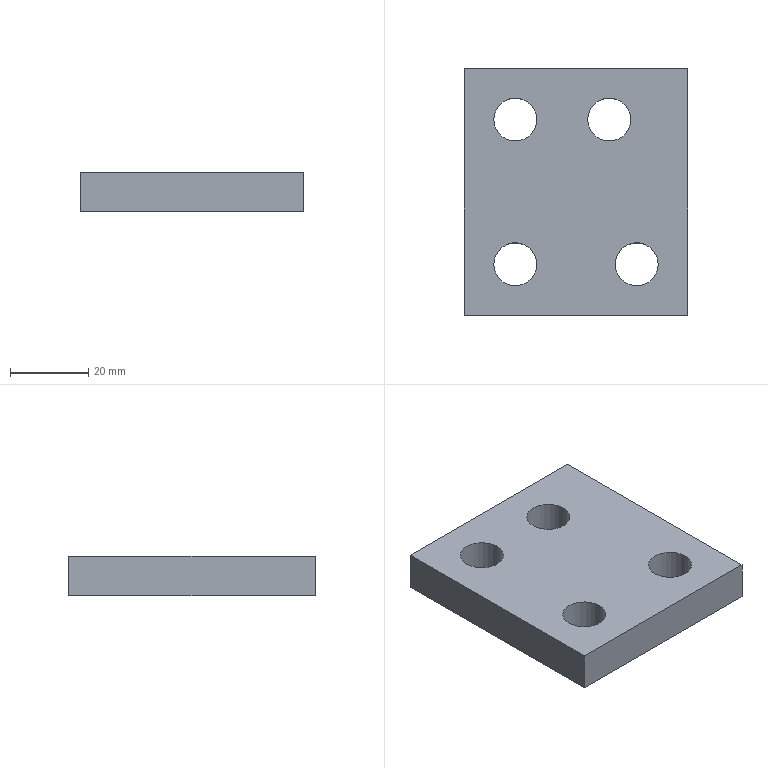Part | NX | features solid 2 | 1 solid | 10 faces | box 57 x 63 x 10 mm | volume 32109 mm3 | plane 6 | cylinder 4 | commonest cylinder face diameters 11 x4
STEP:
#1=CARTESIAN_POINT('',(139.,121.5,88.));
#2=VERTEX_POINT('',#1);
#3=CARTESIAN_POINT('',(133.5,121.5,88.));
#4=DIRECTION('',(0.,0.,1.));
#5=DIRECTION('',(1.,0.,0.));
#6=AXIS2_PLACEMENT_3D('',#3,#4,#5);
#7=CIRCLE('',#6,5.5);
#8=EDGE_CURVE('',#2,#2,#7,.T.);
#9=ORIENTED_EDGE('',*,*,#8,.F.);
#10=EDGE_LOOP('',(#9));
#11=FACE_BOUND('',#10,.T.);
#12=CARTESIAN_POINT('',(163.,158.5,88.));
#13=VERTEX_POINT('',#12);
#14=CARTESIAN_POINT('',(157.5,158.5,88.));
#15=DIRECTION('',(0.,0.,1.));
#16=DIRECTION('',(1.,0.,0.));
#17=AXIS2_PLACEMENT_3D('',#14,#15,#16);
#18=CIRCLE('',#17,5.5);
#19=EDGE_CURVE('',#13,#13,#18,.T.);
#20=ORIENTED_EDGE('',*,*,#19,.F.);
#21=EDGE_LOOP('',(#20));
#22=FACE_BOUND('',#21,.T.);
#23=CARTESIAN_POINT('',(139.,158.5,88.));
#24=VERTEX_POINT('',#23);
#25=CARTESIAN_POINT('',(133.5,158.5,88.));
#26=DIRECTION('',(0.,0.,1.));
#27=DIRECTION('',(1.,0.,0.));
#28=AXIS2_PLACEMENT_3D('',#25,#26,#27);
#29=CIRCLE('',#28,5.5);
#30=EDGE_CURVE('',#24,#24,#29,.T.);
#31=ORIENTED_EDGE('',*,*,#30,.F.);
#32=EDGE_LOOP('',(#31));
#33=FACE_BOUND('',#32,.T.);
#34=CARTESIAN_POINT('',(170.,121.5,88.));
#35=VERTEX_POINT('',#34);
#36=CARTESIAN_POINT('',(164.5,121.5,88.));
#37=DIRECTION('',(0.,0.,1.));
#38=DIRECTION('',(1.,0.,0.));
#39=AXIS2_PLACEMENT_3D('',#36,#37,#38);
#40=CIRCLE('',#39,5.5);
#41=EDGE_CURVE('',#35,#35,#40,.T.);
#42=ORIENTED_EDGE('',*,*,#41,.F.);
#43=EDGE_LOOP('',(#42));
#44=FACE_BOUND('',#43,.T.);
#45=CARTESIAN_POINT('',(177.5,108.5,88.));
#46=VERTEX_POINT('',#45);
#47=CARTESIAN_POINT('',(120.5,108.5,88.));
#48=VERTEX_POINT('',#47);
#49=CARTESIAN_POINT('',(149.,108.5,88.));
#50=DIRECTION('',(-1.,0.,0.));
#51=VECTOR('',#50,1000.);
#52=LINE('',#49,#51);
#53=EDGE_CURVE('',#46,#48,#52,.T.);
#54=ORIENTED_EDGE('',*,*,#53,.F.);
#55=CARTESIAN_POINT('',(177.5,171.5,88.));
#56=VERTEX_POINT('',#55);
#57=CARTESIAN_POINT('',(177.5,140.,88.));
#58=DIRECTION('',(0.,-1.,0.));
#59=VECTOR('',#58,1000.);
#60=LINE('',#57,#59);
#61=EDGE_CURVE('',#56,#46,#60,.T.);
#62=ORIENTED_EDGE('',*,*,#61,.F.);
#63=CARTESIAN_POINT('',(120.5,171.5,88.));
#64=VERTEX_POINT('',#63);
#65=CARTESIAN_POINT('',(149.,171.5,88.));
#66=DIRECTION('',(1.,0.,0.));
#67=VECTOR('',#66,1000.);
#68=LINE('',#65,#67);
#69=EDGE_CURVE('',#64,#56,#68,.T.);
#70=ORIENTED_EDGE('',*,*,#69,.F.);
#71=CARTESIAN_POINT('',(120.5,140.,88.));
#72=DIRECTION('',(0.,1.,0.));
#73=VECTOR('',#72,1000.);
#74=LINE('',#71,#73);
#75=EDGE_CURVE('',#48,#64,#74,.T.);
#76=ORIENTED_EDGE('',*,*,#75,.F.);
#77=EDGE_LOOP('',(#54,#62,#70,#76));
#78=FACE_BOUND('',#77,.T.);
#79=CARTESIAN_POINT('',(268.879,280.,88.));
#80=DIRECTION('',(0.,0.,1.));
#81=DIRECTION('',(-1.,0.,0.));
#82=AXIS2_PLACEMENT_3D('',#79,#80,#81);
#83=PLANE('',#82);
#84=ADVANCED_FACE('',(#11,#22,#33,#44,#78),#83,.T.);
#85=CARTESIAN_POINT('',(177.5,108.5,78.));
#86=VERTEX_POINT('',#85);
#87=CARTESIAN_POINT('',(177.5,108.5,19.));
#88=DIRECTION('',(0.,0.,1.));
#89=VECTOR('',#88,1000.);
#90=LINE('',#87,#89);
#91=EDGE_CURVE('',#86,#46,#90,.T.);
#92=ORIENTED_EDGE('',*,*,#91,.T.);
#93=ORIENTED_EDGE('',*,*,#53,.T.);
#94=CARTESIAN_POINT('',(120.5,108.5,78.));
#95=VERTEX_POINT('',#94);
#96=CARTESIAN_POINT('',(120.5,108.5,19.));
#97=DIRECTION('',(0.,0.,1.));
#98=VECTOR('',#97,1000.);
#99=LINE('',#96,#98);
#100=EDGE_CURVE('',#95,#48,#99,.T.);
#101=ORIENTED_EDGE('',*,*,#100,.F.);
#102=CARTESIAN_POINT('',(149.,108.5,78.));
#103=DIRECTION('',(1.,0.,0.));
#104=VECTOR('',#103,1000.);
#105=LINE('',#102,#104);
#106=EDGE_CURVE('',#95,#86,#105,.T.);
#107=ORIENTED_EDGE('',*,*,#106,.T.);
#108=EDGE_LOOP('',(#92,#93,#101,#107));
#109=FACE_BOUND('',#108,.T.);
#110=CARTESIAN_POINT('',(149.,108.5,19.));
#111=DIRECTION('',(0.,-1.,0.));
#112=DIRECTION('',(0.,0.,-1.));
#113=AXIS2_PLACEMENT_3D('',#110,#111,#112);
#114=PLANE('',#113);
#115=ADVANCED_FACE('',(#109),#114,.T.);
#116=ORIENTED_EDGE('',*,*,#100,.T.);
#117=ORIENTED_EDGE('',*,*,#75,.T.);
#118=CARTESIAN_POINT('',(120.5,171.5,78.));
#119=VERTEX_POINT('',#118);
#120=CARTESIAN_POINT('',(120.5,171.5,19.));
#121=DIRECTION('',(0.,0.,1.));
#122=VECTOR('',#121,1000.);
#123=LINE('',#120,#122);
#124=EDGE_CURVE('',#119,#64,#123,.T.);
#125=ORIENTED_EDGE('',*,*,#124,.F.);
#126=CARTESIAN_POINT('',(120.5,140.,78.));
#127=DIRECTION('',(0.,-1.,0.));
#128=VECTOR('',#127,1000.);
#129=LINE('',#126,#128);
#130=EDGE_CURVE('',#119,#95,#129,.T.);
#131=ORIENTED_EDGE('',*,*,#130,.T.);
#132=EDGE_LOOP('',(#116,#117,#125,#131));
#133=FACE_BOUND('',#132,.T.);
#134=CARTESIAN_POINT('',(120.5,140.,19.));
#135=DIRECTION('',(-1.,0.,0.));
#136=DIRECTION('',(0.,0.,1.));
#137=AXIS2_PLACEMENT_3D('',#134,#135,#136);
#138=PLANE('',#137);
#139=ADVANCED_FACE('',(#133),#138,.T.);
#140=ORIENTED_EDGE('',*,*,#124,.T.);
#141=ORIENTED_EDGE('',*,*,#69,.T.);
#142=CARTESIAN_POINT('',(177.5,171.5,78.));
#143=VERTEX_POINT('',#142);
#144=CARTESIAN_POINT('',(177.5,171.5,19.));
#145=DIRECTION('',(0.,0.,1.));
#146=VECTOR('',#145,1000.);
#147=LINE('',#144,#146);
#148=EDGE_CURVE('',#143,#56,#147,.T.);
#149=ORIENTED_EDGE('',*,*,#148,.F.);
#150=CARTESIAN_POINT('',(149.,171.5,78.));
#151=DIRECTION('',(-1.,0.,0.));
#152=VECTOR('',#151,1000.);
#153=LINE('',#150,#152);
#154=EDGE_CURVE('',#143,#119,#153,.T.);
#155=ORIENTED_EDGE('',*,*,#154,.T.);
#156=EDGE_LOOP('',(#140,#141,#149,#155));
#157=FACE_BOUND('',#156,.T.);
#158=CARTESIAN_POINT('',(149.,171.5,19.));
#159=DIRECTION('',(0.,1.,0.));
#160=DIRECTION('',(0.,0.,1.));
#161=AXIS2_PLACEMENT_3D('',#158,#159,#160);
#162=PLANE('',#161);
#163=ADVANCED_FACE('',(#157),#162,.T.);
#164=CARTESIAN_POINT('',(139.,121.5,78.));
#165=VERTEX_POINT('',#164);
#166=CARTESIAN_POINT('',(133.5,121.5,78.));
#167=DIRECTION('',(0.,0.,1.));
#168=DIRECTION('',(1.,0.,0.));
#169=AXIS2_PLACEMENT_3D('',#166,#167,#168);
#170=CIRCLE('',#169,5.5);
#171=EDGE_CURVE('',#165,#165,#170,.T.);
#172=ORIENTED_EDGE('',*,*,#171,.T.);
#173=EDGE_LOOP('',(#172));
#174=FACE_BOUND('',#173,.T.);
#175=CARTESIAN_POINT('',(163.,158.5,78.));
#176=VERTEX_POINT('',#175);
#177=CARTESIAN_POINT('',(157.5,158.5,78.));
#178=DIRECTION('',(0.,0.,1.));
#179=DIRECTION('',(1.,0.,0.));
#180=AXIS2_PLACEMENT_3D('',#177,#178,#179);
#181=CIRCLE('',#180,5.5);
#182=EDGE_CURVE('',#176,#176,#181,.T.);
#183=ORIENTED_EDGE('',*,*,#182,.T.);
#184=EDGE_LOOP('',(#183));
#185=FACE_BOUND('',#184,.T.);
#186=CARTESIAN_POINT('',(139.,158.5,78.));
#187=VERTEX_POINT('',#186);
#188=CARTESIAN_POINT('',(133.5,158.5,78.));
#189=DIRECTION('',(0.,0.,1.));
#190=DIRECTION('',(1.,0.,0.));
#191=AXIS2_PLACEMENT_3D('',#188,#189,#190);
#192=CIRCLE('',#191,5.5);
#193=EDGE_CURVE('',#187,#187,#192,.T.);
#194=ORIENTED_EDGE('',*,*,#193,.T.);
#195=EDGE_LOOP('',(#194));
#196=FACE_BOUND('',#195,.T.);
#197=CARTESIAN_POINT('',(170.,121.5,78.));
#198=VERTEX_POINT('',#197);
#199=CARTESIAN_POINT('',(164.5,121.5,78.));
#200=DIRECTION('',(0.,0.,1.));
#201=DIRECTION('',(1.,0.,0.));
#202=AXIS2_PLACEMENT_3D('',#199,#200,#201);
#203=CIRCLE('',#202,5.5);
#204=EDGE_CURVE('',#198,#198,#203,.T.);
#205=ORIENTED_EDGE('',*,*,#204,.T.);
#206=EDGE_LOOP('',(#205));
#207=FACE_BOUND('',#206,.T.);
#208=CARTESIAN_POINT('',(177.5,140.,78.));
#209=DIRECTION('',(0.,1.,0.));
#210=VECTOR('',#209,1000.);
#211=LINE('',#208,#210);
#212=EDGE_CURVE('',#86,#143,#211,.T.);
#213=ORIENTED_EDGE('',*,*,#212,.F.);
#214=ORIENTED_EDGE('',*,*,#106,.F.);
#215=ORIENTED_EDGE('',*,*,#130,.F.);
#216=ORIENTED_EDGE('',*,*,#154,.F.);
#217=EDGE_LOOP('',(#213,#214,#215,#216));
#218=FACE_BOUND('',#217,.T.);
#219=CARTESIAN_POINT('',(149.,140.,78.));
#220=DIRECTION('',(0.,0.,-1.));
#221=DIRECTION('',(-1.,0.,0.));
#222=AXIS2_PLACEMENT_3D('',#219,#220,#221);
#223=PLANE('',#222);
#224=ADVANCED_FACE('',(#174,#185,#196,#207,#218),#223,.T.);
#225=ORIENTED_EDGE('',*,*,#212,.T.);
#226=ORIENTED_EDGE('',*,*,#148,.T.);
#227=ORIENTED_EDGE('',*,*,#61,.T.);
#228=ORIENTED_EDGE('',*,*,#91,.F.);
#229=EDGE_LOOP('',(#225,#226,#227,#228));
#230=FACE_BOUND('',#229,.T.);
#231=CARTESIAN_POINT('',(177.5,140.,19.));
#232=DIRECTION('',(1.,0.,0.));
#233=DIRECTION('',(0.,0.,-1.));
#234=AXIS2_PLACEMENT_3D('',#231,#232,#233);
#235=PLANE('',#234);
#236=ADVANCED_FACE('',(#230),#235,.T.);
#237=ORIENTED_EDGE('',*,*,#41,.T.);
#238=EDGE_LOOP('',(#237));
#239=FACE_BOUND('',#238,.T.);
#240=ORIENTED_EDGE('',*,*,#204,.F.);
#241=EDGE_LOOP('',(#240));
#242=FACE_BOUND('',#241,.T.);
#243=CARTESIAN_POINT('',(164.5,121.5,78.));
#244=DIRECTION('',(0.,0.,1.));
#245=DIRECTION('',(1.,0.,0.));
#246=AXIS2_PLACEMENT_3D('',#243,#244,#245);
#247=CYLINDRICAL_SURFACE('',#246,5.5);
#248=ADVANCED_FACE('',(#239,#242),#247,.F.);
#249=ORIENTED_EDGE('',*,*,#30,.T.);
#250=EDGE_LOOP('',(#249));
#251=FACE_BOUND('',#250,.T.);
#252=ORIENTED_EDGE('',*,*,#193,.F.);
#253=EDGE_LOOP('',(#252));
#254=FACE_BOUND('',#253,.T.);
#255=CARTESIAN_POINT('',(133.5,158.5,78.));
#256=DIRECTION('',(0.,0.,1.));
#257=DIRECTION('',(1.,0.,0.));
#258=AXIS2_PLACEMENT_3D('',#255,#256,#257);
#259=CYLINDRICAL_SURFACE('',#258,5.5);
#260=ADVANCED_FACE('',(#251,#254),#259,.F.);
#261=ORIENTED_EDGE('',*,*,#19,.T.);
#262=EDGE_LOOP('',(#261));
#263=FACE_BOUND('',#262,.T.);
#264=ORIENTED_EDGE('',*,*,#182,.F.);
#265=EDGE_LOOP('',(#264));
#266=FACE_BOUND('',#265,.T.);
#267=CARTESIAN_POINT('',(157.5,158.5,78.));
#268=DIRECTION('',(0.,0.,1.));
#269=DIRECTION('',(1.,0.,0.));
#270=AXIS2_PLACEMENT_3D('',#267,#268,#269);
#271=CYLINDRICAL_SURFACE('',#270,5.5);
#272=ADVANCED_FACE('',(#263,#266),#271,.F.);
#273=ORIENTED_EDGE('',*,*,#8,.T.);
#274=EDGE_LOOP('',(#273));
#275=FACE_BOUND('',#274,.T.);
#276=ORIENTED_EDGE('',*,*,#171,.F.);
#277=EDGE_LOOP('',(#276));
#278=FACE_BOUND('',#277,.T.);
#279=CARTESIAN_POINT('',(133.5,121.5,78.));
#280=DIRECTION('',(0.,0.,1.));
#281=DIRECTION('',(1.,0.,0.));
#282=AXIS2_PLACEMENT_3D('',#279,#280,#281);
#283=CYLINDRICAL_SURFACE('',#282,5.5);
#284=ADVANCED_FACE('',(#275,#278),#283,.F.);
#285=CLOSED_SHELL('',(#84,#115,#139,#163,#224,#236,#248,#260,#272,#284));
#286=MANIFOLD_SOLID_BREP('',#285);
#287=(LENGTH_UNIT()NAMED_UNIT(*)SI_UNIT(.MILLI.,.METRE.));
#288=UNCERTAINTY_MEASURE_WITH_UNIT(LENGTH_MEASURE(0.00001),#287,'','');
#289=(NAMED_UNIT(*)PLANE_ANGLE_UNIT()SI_UNIT($,.RADIAN.));
#290=(NAMED_UNIT(*)SI_UNIT($,.STERADIAN.)SOLID_ANGLE_UNIT());
#291=(GEOMETRIC_REPRESENTATION_CONTEXT(3)GLOBAL_UNCERTAINTY_ASSIGNED_CONTEXT((#288))GLOBAL_UNIT_ASSIGNED_CONTEXT((#287,#289,#290))REPRESENTATION_CONTEXT('',''));
#292=ADVANCED_BREP_SHAPE_REPRESENTATION('',(#286),#291);